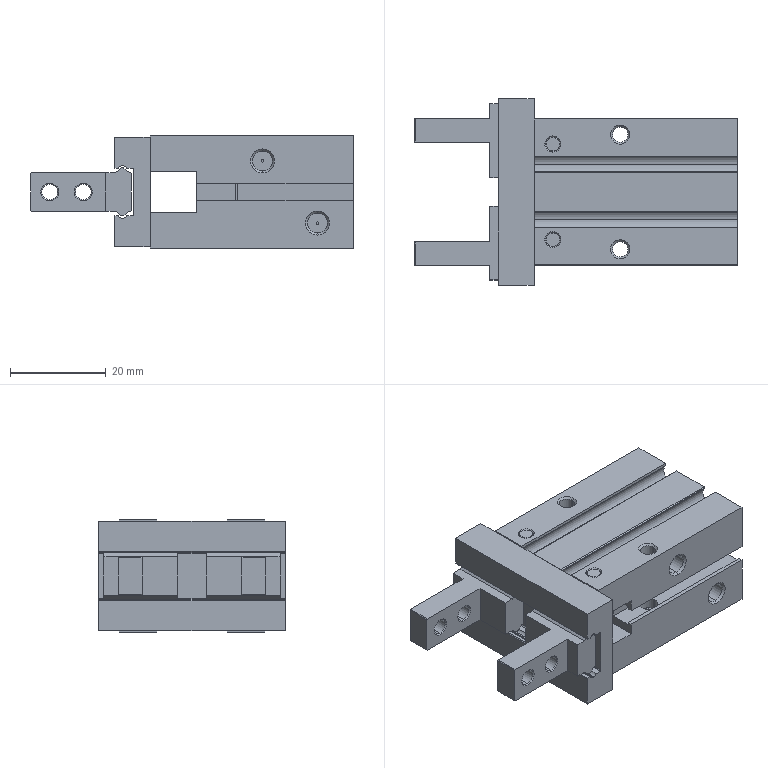Part | SolidWorks | 3 solids | 249 faces | box 67.5 x 39 x 23.5 mm | volume 30109 mm3 | plane 116 | cylinder 71 | cone 62 | commonest cylinder face diameters 3.242 x16 0.4 x10 3.3 x8 1 x6 4.02 x6 4.2 x6